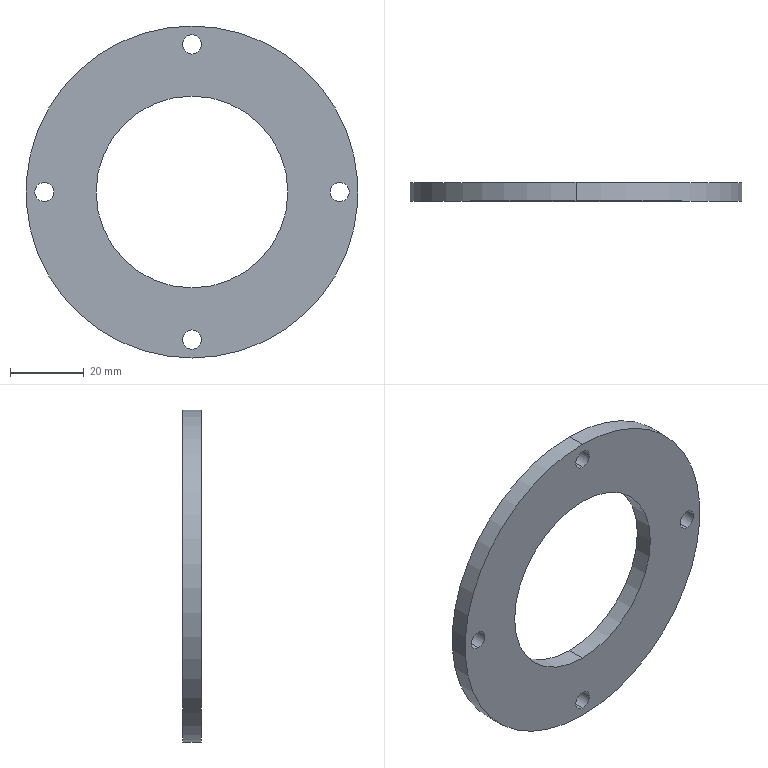Part | NX | features BREP 1 | 1 solid | 14 faces | box 90 x 5 x 90 mm | volume 20765 mm3 | cylinder 12 | plane 2 | commonest cylinder face diameters 5.2 x8 52 x2 90 x2
STEP:
#1=CARTESIAN_POINT('',(-40.,0.,-2.6));
#2=VERTEX_POINT('',#1);
#3=CARTESIAN_POINT('',(-40.,0.,2.6));
#4=VERTEX_POINT('',#3);
#5=CARTESIAN_POINT('',(-40.,0.,0.));
#6=DIRECTION('',(0.,1.,0.));
#7=DIRECTION('',(0.,0.,1.));
#8=AXIS2_PLACEMENT_3D('',#5,#6,#7);
#9=CIRCLE('',#8,2.6);
#10=EDGE_CURVE('',#2,#4,#9,.T.);
#11=ORIENTED_EDGE('',*,*,#10,.F.);
#12=CARTESIAN_POINT('',(-40.,5.,-2.6));
#13=VERTEX_POINT('',#12);
#14=CARTESIAN_POINT('',(-40.,-5.,-2.6));
#15=DIRECTION('',(0.,1.,0.));
#16=VECTOR('',#15,1000.);
#17=LINE('',#14,#16);
#18=EDGE_CURVE('',#2,#13,#17,.T.);
#19=ORIENTED_EDGE('',*,*,#18,.T.);
#20=CARTESIAN_POINT('',(-40.,5.,2.6));
#21=VERTEX_POINT('',#20);
#22=CARTESIAN_POINT('',(-40.,5.,0.));
#23=DIRECTION('',(0.,1.,0.));
#24=DIRECTION('',(0.,0.,1.));
#25=AXIS2_PLACEMENT_3D('',#22,#23,#24);
#26=CIRCLE('',#25,2.6);
#27=EDGE_CURVE('',#13,#21,#26,.T.);
#28=ORIENTED_EDGE('',*,*,#27,.T.);
#29=CARTESIAN_POINT('',(-40.,-5.,2.6));
#30=DIRECTION('',(0.,1.,0.));
#31=VECTOR('',#30,1000.);
#32=LINE('',#29,#31);
#33=EDGE_CURVE('',#4,#21,#32,.T.);
#34=ORIENTED_EDGE('',*,*,#33,.F.);
#35=EDGE_LOOP('',(#11,#19,#28,#34));
#36=FACE_BOUND('',#35,.T.);
#37=CARTESIAN_POINT('',(-40.,-5.,0.));
#38=DIRECTION('',(0.,1.,0.));
#39=DIRECTION('',(0.,0.,-1.));
#40=AXIS2_PLACEMENT_3D('',#37,#38,#39);
#41=CYLINDRICAL_SURFACE('',#40,2.6);
#42=ADVANCED_FACE('',(#36),#41,.F.);
#43=CARTESIAN_POINT('',(0.,0.,-42.6));
#44=VERTEX_POINT('',#43);
#45=CARTESIAN_POINT('',(0.,0.,-37.4));
#46=VERTEX_POINT('',#45);
#47=CARTESIAN_POINT('',(0.,0.,-40.));
#48=DIRECTION('',(0.,1.,0.));
#49=DIRECTION('',(0.,0.,1.));
#50=AXIS2_PLACEMENT_3D('',#47,#48,#49);
#51=CIRCLE('',#50,2.6);
#52=EDGE_CURVE('',#44,#46,#51,.T.);
#53=ORIENTED_EDGE('',*,*,#52,.F.);
#54=CARTESIAN_POINT('',(0.,5.,-42.6));
#55=VERTEX_POINT('',#54);
#56=CARTESIAN_POINT('',(0.,-5.,-42.6));
#57=DIRECTION('',(0.,1.,0.));
#58=VECTOR('',#57,1000.);
#59=LINE('',#56,#58);
#60=EDGE_CURVE('',#44,#55,#59,.T.);
#61=ORIENTED_EDGE('',*,*,#60,.T.);
#62=CARTESIAN_POINT('',(0.,5.,-37.4));
#63=VERTEX_POINT('',#62);
#64=CARTESIAN_POINT('',(0.,5.,-40.));
#65=DIRECTION('',(0.,1.,0.));
#66=DIRECTION('',(0.,0.,1.));
#67=AXIS2_PLACEMENT_3D('',#64,#65,#66);
#68=CIRCLE('',#67,2.6);
#69=EDGE_CURVE('',#55,#63,#68,.T.);
#70=ORIENTED_EDGE('',*,*,#69,.T.);
#71=CARTESIAN_POINT('',(0.,-5.,-37.4));
#72=DIRECTION('',(0.,1.,0.));
#73=VECTOR('',#72,1000.);
#74=LINE('',#71,#73);
#75=EDGE_CURVE('',#46,#63,#74,.T.);
#76=ORIENTED_EDGE('',*,*,#75,.F.);
#77=EDGE_LOOP('',(#53,#61,#70,#76));
#78=FACE_BOUND('',#77,.T.);
#79=CARTESIAN_POINT('',(0.,-5.,-40.));
#80=DIRECTION('',(0.,1.,0.));
#81=DIRECTION('',(0.,0.,-1.));
#82=AXIS2_PLACEMENT_3D('',#79,#80,#81);
#83=CYLINDRICAL_SURFACE('',#82,2.6);
#84=ADVANCED_FACE('',(#78),#83,.F.);
#85=CARTESIAN_POINT('',(40.,0.,-2.6));
#86=VERTEX_POINT('',#85);
#87=CARTESIAN_POINT('',(40.,0.,2.6));
#88=VERTEX_POINT('',#87);
#89=CARTESIAN_POINT('',(40.,0.,0.));
#90=DIRECTION('',(0.,1.,0.));
#91=DIRECTION('',(0.,0.,1.));
#92=AXIS2_PLACEMENT_3D('',#89,#90,#91);
#93=CIRCLE('',#92,2.6);
#94=EDGE_CURVE('',#86,#88,#93,.T.);
#95=ORIENTED_EDGE('',*,*,#94,.F.);
#96=CARTESIAN_POINT('',(40.,5.,-2.6));
#97=VERTEX_POINT('',#96);
#98=CARTESIAN_POINT('',(40.,-5.,-2.6));
#99=DIRECTION('',(0.,1.,0.));
#100=VECTOR('',#99,1000.);
#101=LINE('',#98,#100);
#102=EDGE_CURVE('',#86,#97,#101,.T.);
#103=ORIENTED_EDGE('',*,*,#102,.T.);
#104=CARTESIAN_POINT('',(40.,5.,2.6));
#105=VERTEX_POINT('',#104);
#106=CARTESIAN_POINT('',(40.,5.,0.));
#107=DIRECTION('',(0.,1.,0.));
#108=DIRECTION('',(0.,0.,1.));
#109=AXIS2_PLACEMENT_3D('',#106,#107,#108);
#110=CIRCLE('',#109,2.6);
#111=EDGE_CURVE('',#97,#105,#110,.T.);
#112=ORIENTED_EDGE('',*,*,#111,.T.);
#113=CARTESIAN_POINT('',(40.,-5.,2.6));
#114=DIRECTION('',(0.,1.,0.));
#115=VECTOR('',#114,1000.);
#116=LINE('',#113,#115);
#117=EDGE_CURVE('',#88,#105,#116,.T.);
#118=ORIENTED_EDGE('',*,*,#117,.F.);
#119=EDGE_LOOP('',(#95,#103,#112,#118));
#120=FACE_BOUND('',#119,.T.);
#121=CARTESIAN_POINT('',(40.,-5.,0.));
#122=DIRECTION('',(0.,1.,0.));
#123=DIRECTION('',(0.,0.,-1.));
#124=AXIS2_PLACEMENT_3D('',#121,#122,#123);
#125=CYLINDRICAL_SURFACE('',#124,2.6);
#126=ADVANCED_FACE('',(#120),#125,.F.);
#127=CARTESIAN_POINT('',(0.,0.,37.4));
#128=VERTEX_POINT('',#127);
#129=CARTESIAN_POINT('',(0.,0.,42.6));
#130=VERTEX_POINT('',#129);
#131=CARTESIAN_POINT('',(0.,0.,40.));
#132=DIRECTION('',(0.,1.,0.));
#133=DIRECTION('',(0.,0.,1.));
#134=AXIS2_PLACEMENT_3D('',#131,#132,#133);
#135=CIRCLE('',#134,2.6);
#136=EDGE_CURVE('',#128,#130,#135,.T.);
#137=ORIENTED_EDGE('',*,*,#136,.F.);
#138=CARTESIAN_POINT('',(0.,5.,37.4));
#139=VERTEX_POINT('',#138);
#140=CARTESIAN_POINT('',(0.,-5.,37.4));
#141=DIRECTION('',(0.,1.,0.));
#142=VECTOR('',#141,1000.);
#143=LINE('',#140,#142);
#144=EDGE_CURVE('',#128,#139,#143,.T.);
#145=ORIENTED_EDGE('',*,*,#144,.T.);
#146=CARTESIAN_POINT('',(0.,5.,42.6));
#147=VERTEX_POINT('',#146);
#148=CARTESIAN_POINT('',(0.,5.,40.));
#149=DIRECTION('',(0.,1.,0.));
#150=DIRECTION('',(0.,0.,1.));
#151=AXIS2_PLACEMENT_3D('',#148,#149,#150);
#152=CIRCLE('',#151,2.6);
#153=EDGE_CURVE('',#139,#147,#152,.T.);
#154=ORIENTED_EDGE('',*,*,#153,.T.);
#155=CARTESIAN_POINT('',(0.,-5.,42.6));
#156=DIRECTION('',(0.,1.,0.));
#157=VECTOR('',#156,1000.);
#158=LINE('',#155,#157);
#159=EDGE_CURVE('',#130,#147,#158,.T.);
#160=ORIENTED_EDGE('',*,*,#159,.F.);
#161=EDGE_LOOP('',(#137,#145,#154,#160));
#162=FACE_BOUND('',#161,.T.);
#163=CARTESIAN_POINT('',(0.,-5.,40.));
#164=DIRECTION('',(0.,1.,0.));
#165=DIRECTION('',(0.,0.,-1.));
#166=AXIS2_PLACEMENT_3D('',#163,#164,#165);
#167=CYLINDRICAL_SURFACE('',#166,2.6);
#168=ADVANCED_FACE('',(#162),#167,.F.);
#169=CARTESIAN_POINT('',(0.,5.,-26.));
#170=VERTEX_POINT('',#169);
#171=CARTESIAN_POINT('',(0.,5.,26.));
#172=VERTEX_POINT('',#171);
#173=CARTESIAN_POINT('',(0.,5.,0.));
#174=DIRECTION('',(0.,1.,0.));
#175=DIRECTION('',(0.,0.,1.));
#176=AXIS2_PLACEMENT_3D('',#173,#174,#175);
#177=CIRCLE('',#176,26.);
#178=EDGE_CURVE('',#170,#172,#177,.T.);
#179=ORIENTED_EDGE('',*,*,#178,.T.);
#180=CARTESIAN_POINT('',(0.,0.,26.));
#181=VERTEX_POINT('',#180);
#182=CARTESIAN_POINT('',(0.,5.,26.));
#183=DIRECTION('',(0.,-1.,0.));
#184=VECTOR('',#183,1000.);
#185=LINE('',#182,#184);
#186=EDGE_CURVE('',#181,#172,#185,.F.);
#187=ORIENTED_EDGE('',*,*,#186,.F.);
#188=CARTESIAN_POINT('',(0.,0.,-26.));
#189=VERTEX_POINT('',#188);
#190=CARTESIAN_POINT('',(0.,0.,0.));
#191=DIRECTION('',(0.,1.,0.));
#192=DIRECTION('',(0.,0.,1.));
#193=AXIS2_PLACEMENT_3D('',#190,#191,#192);
#194=CIRCLE('',#193,26.);
#195=EDGE_CURVE('',#189,#181,#194,.T.);
#196=ORIENTED_EDGE('',*,*,#195,.F.);
#197=CARTESIAN_POINT('',(0.,5.,-26.));
#198=DIRECTION('',(0.,-1.,0.));
#199=VECTOR('',#198,1000.);
#200=LINE('',#197,#199);
#201=EDGE_CURVE('',#189,#170,#200,.F.);
#202=ORIENTED_EDGE('',*,*,#201,.T.);
#203=EDGE_LOOP('',(#179,#187,#196,#202));
#204=FACE_BOUND('',#203,.T.);
#205=CARTESIAN_POINT('',(0.,5.,0.));
#206=DIRECTION('',(0.,-1.,0.));
#207=DIRECTION('',(0.,0.,1.));
#208=AXIS2_PLACEMENT_3D('',#205,#206,#207);
#209=CYLINDRICAL_SURFACE('',#208,26.);
#210=ADVANCED_FACE('',(#204),#209,.F.);
#211=CARTESIAN_POINT('',(0.,5.,45.));
#212=VERTEX_POINT('',#211);
#213=CARTESIAN_POINT('',(0.,5.,-45.));
#214=VERTEX_POINT('',#213);
#215=CARTESIAN_POINT('',(0.,5.,0.));
#216=DIRECTION('',(0.,1.,0.));
#217=DIRECTION('',(0.,0.,1.));
#218=AXIS2_PLACEMENT_3D('',#215,#216,#217);
#219=CIRCLE('',#218,45.);
#220=EDGE_CURVE('',#212,#214,#219,.T.);
#221=ORIENTED_EDGE('',*,*,#220,.F.);
#222=CARTESIAN_POINT('',(0.,0.,45.));
#223=VERTEX_POINT('',#222);
#224=CARTESIAN_POINT('',(0.,5.,45.));
#225=DIRECTION('',(0.,-1.,0.));
#226=VECTOR('',#225,1000.);
#227=LINE('',#224,#226);
#228=EDGE_CURVE('',#223,#212,#227,.F.);
#229=ORIENTED_EDGE('',*,*,#228,.F.);
#230=CARTESIAN_POINT('',(0.,0.,-45.));
#231=VERTEX_POINT('',#230);
#232=CARTESIAN_POINT('',(0.,0.,0.));
#233=DIRECTION('',(0.,1.,0.));
#234=DIRECTION('',(0.,0.,1.));
#235=AXIS2_PLACEMENT_3D('',#232,#233,#234);
#236=CIRCLE('',#235,45.);
#237=EDGE_CURVE('',#223,#231,#236,.T.);
#238=ORIENTED_EDGE('',*,*,#237,.T.);
#239=CARTESIAN_POINT('',(0.,5.,-45.));
#240=DIRECTION('',(0.,-1.,0.));
#241=VECTOR('',#240,1000.);
#242=LINE('',#239,#241);
#243=EDGE_CURVE('',#231,#214,#242,.F.);
#244=ORIENTED_EDGE('',*,*,#243,.T.);
#245=EDGE_LOOP('',(#221,#229,#238,#244));
#246=FACE_BOUND('',#245,.T.);
#247=CARTESIAN_POINT('',(0.,5.,0.));
#248=DIRECTION('',(0.,-1.,0.));
#249=DIRECTION('',(0.,0.,1.));
#250=AXIS2_PLACEMENT_3D('',#247,#248,#249);
#251=CYLINDRICAL_SURFACE('',#250,45.);
#252=ADVANCED_FACE('',(#246),#251,.T.);
#253=CARTESIAN_POINT('',(0.,5.,0.));
#254=DIRECTION('',(0.,1.,0.));
#255=DIRECTION('',(0.,0.,1.));
#256=AXIS2_PLACEMENT_3D('',#253,#254,#255);
#257=CIRCLE('',#256,45.);
#258=EDGE_CURVE('',#214,#212,#257,.T.);
#259=ORIENTED_EDGE('',*,*,#258,.T.);
#260=ORIENTED_EDGE('',*,*,#220,.T.);
#261=EDGE_LOOP('',(#259,#260));
#262=FACE_BOUND('',#261,.T.);
#263=CARTESIAN_POINT('',(-40.,5.,0.));
#264=DIRECTION('',(0.,1.,0.));
#265=DIRECTION('',(0.,0.,1.));
#266=AXIS2_PLACEMENT_3D('',#263,#264,#265);
#267=CIRCLE('',#266,2.6);
#268=EDGE_CURVE('',#21,#13,#267,.T.);
#269=ORIENTED_EDGE('',*,*,#268,.F.);
#270=ORIENTED_EDGE('',*,*,#27,.F.);
#271=EDGE_LOOP('',(#269,#270));
#272=FACE_BOUND('',#271,.T.);
#273=CARTESIAN_POINT('',(0.,5.,-40.));
#274=DIRECTION('',(0.,1.,0.));
#275=DIRECTION('',(0.,0.,1.));
#276=AXIS2_PLACEMENT_3D('',#273,#274,#275);
#277=CIRCLE('',#276,2.6);
#278=EDGE_CURVE('',#63,#55,#277,.T.);
#279=ORIENTED_EDGE('',*,*,#278,.F.);
#280=ORIENTED_EDGE('',*,*,#69,.F.);
#281=EDGE_LOOP('',(#279,#280));
#282=FACE_BOUND('',#281,.T.);
#283=CARTESIAN_POINT('',(40.,5.,0.));
#284=DIRECTION('',(0.,1.,0.));
#285=DIRECTION('',(0.,0.,1.));
#286=AXIS2_PLACEMENT_3D('',#283,#284,#285);
#287=CIRCLE('',#286,2.6);
#288=EDGE_CURVE('',#105,#97,#287,.T.);
#289=ORIENTED_EDGE('',*,*,#288,.F.);
#290=ORIENTED_EDGE('',*,*,#111,.F.);
#291=EDGE_LOOP('',(#289,#290));
#292=FACE_BOUND('',#291,.T.);
#293=CARTESIAN_POINT('',(0.,5.,40.));
#294=DIRECTION('',(0.,1.,0.));
#295=DIRECTION('',(0.,0.,1.));
#296=AXIS2_PLACEMENT_3D('',#293,#294,#295);
#297=CIRCLE('',#296,2.6);
#298=EDGE_CURVE('',#147,#139,#297,.T.);
#299=ORIENTED_EDGE('',*,*,#298,.F.);
#300=ORIENTED_EDGE('',*,*,#153,.F.);
#301=EDGE_LOOP('',(#299,#300));
#302=FACE_BOUND('',#301,.T.);
#303=ORIENTED_EDGE('',*,*,#178,.F.);
#304=CARTESIAN_POINT('',(0.,5.,0.));
#305=DIRECTION('',(0.,1.,0.));
#306=DIRECTION('',(0.,0.,1.));
#307=AXIS2_PLACEMENT_3D('',#304,#305,#306);
#308=CIRCLE('',#307,26.);
#309=EDGE_CURVE('',#172,#170,#308,.T.);
#310=ORIENTED_EDGE('',*,*,#309,.F.);
#311=EDGE_LOOP('',(#303,#310));
#312=FACE_BOUND('',#311,.T.);
#313=CARTESIAN_POINT('',(0.,5.,0.));
#314=DIRECTION('',(0.,1.,0.));
#315=DIRECTION('',(0.,0.,1.));
#316=AXIS2_PLACEMENT_3D('',#313,#314,#315);
#317=PLANE('',#316);
#318=ADVANCED_FACE('',(#262,#272,#282,#292,#302,#312),#317,.T.);
#319=CARTESIAN_POINT('',(0.,0.,0.));
#320=DIRECTION('',(0.,1.,0.));
#321=DIRECTION('',(0.,0.,1.));
#322=AXIS2_PLACEMENT_3D('',#319,#320,#321);
#323=CIRCLE('',#322,45.);
#324=EDGE_CURVE('',#231,#223,#323,.T.);
#325=ORIENTED_EDGE('',*,*,#324,.F.);
#326=ORIENTED_EDGE('',*,*,#237,.F.);
#327=EDGE_LOOP('',(#325,#326));
#328=FACE_BOUND('',#327,.T.);
#329=CARTESIAN_POINT('',(-40.,0.,0.));
#330=DIRECTION('',(0.,1.,0.));
#331=DIRECTION('',(0.,0.,1.));
#332=AXIS2_PLACEMENT_3D('',#329,#330,#331);
#333=CIRCLE('',#332,2.6);
#334=EDGE_CURVE('',#4,#2,#333,.T.);
#335=ORIENTED_EDGE('',*,*,#334,.T.);
#336=ORIENTED_EDGE('',*,*,#10,.T.);
#337=EDGE_LOOP('',(#335,#336));
#338=FACE_BOUND('',#337,.T.);
#339=CARTESIAN_POINT('',(0.,0.,-40.));
#340=DIRECTION('',(0.,1.,0.));
#341=DIRECTION('',(0.,0.,1.));
#342=AXIS2_PLACEMENT_3D('',#339,#340,#341);
#343=CIRCLE('',#342,2.6);
#344=EDGE_CURVE('',#46,#44,#343,.T.);
#345=ORIENTED_EDGE('',*,*,#344,.T.);
#346=ORIENTED_EDGE('',*,*,#52,.T.);
#347=EDGE_LOOP('',(#345,#346));
#348=FACE_BOUND('',#347,.T.);
#349=CARTESIAN_POINT('',(40.,0.,0.));
#350=DIRECTION('',(0.,1.,0.));
#351=DIRECTION('',(0.,0.,1.));
#352=AXIS2_PLACEMENT_3D('',#349,#350,#351);
#353=CIRCLE('',#352,2.6);
#354=EDGE_CURVE('',#88,#86,#353,.T.);
#355=ORIENTED_EDGE('',*,*,#354,.T.);
#356=ORIENTED_EDGE('',*,*,#94,.T.);
#357=EDGE_LOOP('',(#355,#356));
#358=FACE_BOUND('',#357,.T.);
#359=CARTESIAN_POINT('',(0.,0.,40.));
#360=DIRECTION('',(0.,1.,0.));
#361=DIRECTION('',(0.,0.,1.));
#362=AXIS2_PLACEMENT_3D('',#359,#360,#361);
#363=CIRCLE('',#362,2.6);
#364=EDGE_CURVE('',#130,#128,#363,.T.);
#365=ORIENTED_EDGE('',*,*,#364,.T.);
#366=ORIENTED_EDGE('',*,*,#136,.T.);
#367=EDGE_LOOP('',(#365,#366));
#368=FACE_BOUND('',#367,.T.);
#369=ORIENTED_EDGE('',*,*,#195,.T.);
#370=CARTESIAN_POINT('',(0.,0.,0.));
#371=DIRECTION('',(0.,1.,0.));
#372=DIRECTION('',(0.,0.,1.));
#373=AXIS2_PLACEMENT_3D('',#370,#371,#372);
#374=CIRCLE('',#373,26.);
#375=EDGE_CURVE('',#181,#189,#374,.T.);
#376=ORIENTED_EDGE('',*,*,#375,.T.);
#377=EDGE_LOOP('',(#369,#376));
#378=FACE_BOUND('',#377,.T.);
#379=CARTESIAN_POINT('',(0.,0.,0.));
#380=DIRECTION('',(0.,1.,0.));
#381=DIRECTION('',(0.,0.,1.));
#382=AXIS2_PLACEMENT_3D('',#379,#380,#381);
#383=PLANE('',#382);
#384=ADVANCED_FACE('',(#328,#338,#348,#358,#368,#378),#383,.F.);
#385=ORIENTED_EDGE('',*,*,#228,.T.);
#386=ORIENTED_EDGE('',*,*,#258,.F.);
#387=ORIENTED_EDGE('',*,*,#243,.F.);
#388=ORIENTED_EDGE('',*,*,#324,.T.);
#389=EDGE_LOOP('',(#385,#386,#387,#388));
#390=FACE_BOUND('',#389,.T.);
#391=CARTESIAN_POINT('',(0.,5.,0.));
#392=DIRECTION('',(0.,-1.,0.));
#393=DIRECTION('',(0.,0.,1.));
#394=AXIS2_PLACEMENT_3D('',#391,#392,#393);
#395=CYLINDRICAL_SURFACE('',#394,45.);
#396=ADVANCED_FACE('',(#390),#395,.T.);
#397=ORIENTED_EDGE('',*,*,#186,.T.);
#398=ORIENTED_EDGE('',*,*,#309,.T.);
#399=ORIENTED_EDGE('',*,*,#201,.F.);
#400=ORIENTED_EDGE('',*,*,#375,.F.);
#401=EDGE_LOOP('',(#397,#398,#399,#400));
#402=FACE_BOUND('',#401,.T.);
#403=CARTESIAN_POINT('',(0.,5.,0.));
#404=DIRECTION('',(0.,-1.,0.));
#405=DIRECTION('',(0.,0.,1.));
#406=AXIS2_PLACEMENT_3D('',#403,#404,#405);
#407=CYLINDRICAL_SURFACE('',#406,26.);
#408=ADVANCED_FACE('',(#402),#407,.F.);
#409=ORIENTED_EDGE('',*,*,#144,.F.);
#410=ORIENTED_EDGE('',*,*,#364,.F.);
#411=ORIENTED_EDGE('',*,*,#159,.T.);
#412=ORIENTED_EDGE('',*,*,#298,.T.);
#413=EDGE_LOOP('',(#409,#410,#411,#412));
#414=FACE_BOUND('',#413,.T.);
#415=CARTESIAN_POINT('',(0.,-5.,40.));
#416=DIRECTION('',(0.,1.,0.));
#417=DIRECTION('',(0.,0.,-1.));
#418=AXIS2_PLACEMENT_3D('',#415,#416,#417);
#419=CYLINDRICAL_SURFACE('',#418,2.6);
#420=ADVANCED_FACE('',(#414),#419,.F.);
#421=ORIENTED_EDGE('',*,*,#102,.F.);
#422=ORIENTED_EDGE('',*,*,#354,.F.);
#423=ORIENTED_EDGE('',*,*,#117,.T.);
#424=ORIENTED_EDGE('',*,*,#288,.T.);
#425=EDGE_LOOP('',(#421,#422,#423,#424));
#426=FACE_BOUND('',#425,.T.);
#427=CARTESIAN_POINT('',(40.,-5.,0.));
#428=DIRECTION('',(0.,1.,0.));
#429=DIRECTION('',(0.,0.,-1.));
#430=AXIS2_PLACEMENT_3D('',#427,#428,#429);
#431=CYLINDRICAL_SURFACE('',#430,2.6);
#432=ADVANCED_FACE('',(#426),#431,.F.);
#433=ORIENTED_EDGE('',*,*,#60,.F.);
#434=ORIENTED_EDGE('',*,*,#344,.F.);
#435=ORIENTED_EDGE('',*,*,#75,.T.);
#436=ORIENTED_EDGE('',*,*,#278,.T.);
#437=EDGE_LOOP('',(#433,#434,#435,#436));
#438=FACE_BOUND('',#437,.T.);
#439=CARTESIAN_POINT('',(0.,-5.,-40.));
#440=DIRECTION('',(0.,1.,0.));
#441=DIRECTION('',(0.,0.,-1.));
#442=AXIS2_PLACEMENT_3D('',#439,#440,#441);
#443=CYLINDRICAL_SURFACE('',#442,2.6);
#444=ADVANCED_FACE('',(#438),#443,.F.);
#445=ORIENTED_EDGE('',*,*,#18,.F.);
#446=ORIENTED_EDGE('',*,*,#334,.F.);
#447=ORIENTED_EDGE('',*,*,#33,.T.);
#448=ORIENTED_EDGE('',*,*,#268,.T.);
#449=EDGE_LOOP('',(#445,#446,#447,#448));
#450=FACE_BOUND('',#449,.T.);
#451=CARTESIAN_POINT('',(-40.,-5.,0.));
#452=DIRECTION('',(0.,1.,0.));
#453=DIRECTION('',(0.,0.,-1.));
#454=AXIS2_PLACEMENT_3D('',#451,#452,#453);
#455=CYLINDRICAL_SURFACE('',#454,2.6);
#456=ADVANCED_FACE('',(#450),#455,.F.);
#457=CLOSED_SHELL('',(#42,#84,#126,#168,#210,#252,#318,#384,#396,#408,#420,#432,#444,#456));
#458=MANIFOLD_SOLID_BREP('',#457);
#459=(LENGTH_UNIT()NAMED_UNIT(*)SI_UNIT(.MILLI.,.METRE.));
#460=UNCERTAINTY_MEASURE_WITH_UNIT(LENGTH_MEASURE(0.00001),#459,'','');
#461=(NAMED_UNIT(*)PLANE_ANGLE_UNIT()SI_UNIT($,.RADIAN.));
#462=(NAMED_UNIT(*)SI_UNIT($,.STERADIAN.)SOLID_ANGLE_UNIT());
#463=(GEOMETRIC_REPRESENTATION_CONTEXT(3)GLOBAL_UNCERTAINTY_ASSIGNED_CONTEXT((#460))GLOBAL_UNIT_ASSIGNED_CONTEXT((#459,#461,#462))REPRESENTATION_CONTEXT('',''));
#464=ADVANCED_BREP_SHAPE_REPRESENTATION('',(#458),#463);